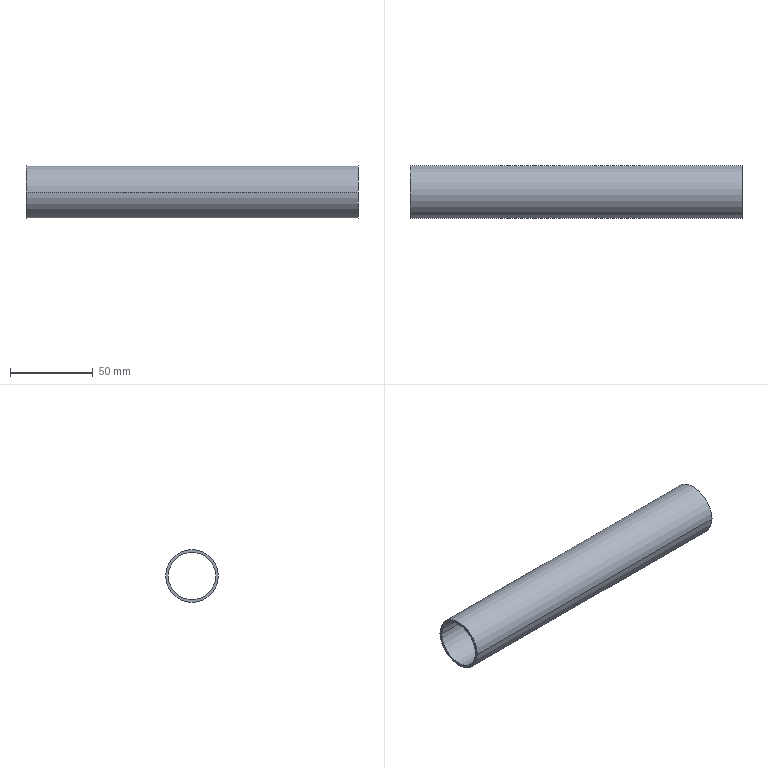Part | NX | features BREP 1 | 1 solid | 6 faces | box 200.025 x 31.75 x 31.75 mm | volume 30090 mm3 | cylinder 4 | plane 2 | commonest cylinder face diameters 28.575 x2 31.75 x2
STEP:
#1=CARTESIAN_POINT('',(-100.013,15.875,0.));
#2=VERTEX_POINT('',#1);
#3=CARTESIAN_POINT('',(-100.013,-15.875,0.));
#4=VERTEX_POINT('',#3);
#5=CARTESIAN_POINT('',(-100.013,0.,0.));
#6=DIRECTION('',(1.,0.,0.));
#7=DIRECTION('',(0.,1.,0.));
#8=AXIS2_PLACEMENT_3D('',#5,#6,#7);
#9=CIRCLE('',#8,15.875);
#10=EDGE_CURVE('',#2,#4,#9,.T.);
#11=ORIENTED_EDGE('',*,*,#10,.F.);
#12=CARTESIAN_POINT('',(-100.013,0.,0.));
#13=DIRECTION('',(1.,0.,0.));
#14=DIRECTION('',(0.,-1.,0.));
#15=AXIS2_PLACEMENT_3D('',#12,#13,#14);
#16=CIRCLE('',#15,15.875);
#17=EDGE_CURVE('',#4,#2,#16,.T.);
#18=ORIENTED_EDGE('',*,*,#17,.F.);
#19=EDGE_LOOP('',(#11,#18));
#20=FACE_BOUND('',#19,.T.);
#21=CARTESIAN_POINT('',(-100.013,14.287,0.));
#22=VERTEX_POINT('',#21);
#23=CARTESIAN_POINT('',(-100.013,-14.287,0.));
#24=VERTEX_POINT('',#23);
#25=CARTESIAN_POINT('',(-100.013,0.,0.));
#26=DIRECTION('',(-1.,0.,0.));
#27=DIRECTION('',(0.,1.,0.));
#28=AXIS2_PLACEMENT_3D('',#25,#26,#27);
#29=CIRCLE('',#28,14.287);
#30=EDGE_CURVE('',#22,#24,#29,.T.);
#31=ORIENTED_EDGE('',*,*,#30,.F.);
#32=CARTESIAN_POINT('',(-100.013,0.,0.));
#33=DIRECTION('',(-1.,0.,0.));
#34=DIRECTION('',(0.,-1.,0.));
#35=AXIS2_PLACEMENT_3D('',#32,#33,#34);
#36=CIRCLE('',#35,14.287);
#37=EDGE_CURVE('',#24,#22,#36,.T.);
#38=ORIENTED_EDGE('',*,*,#37,.F.);
#39=EDGE_LOOP('',(#31,#38));
#40=FACE_BOUND('',#39,.T.);
#41=CARTESIAN_POINT('',(-100.013,0.,0.));
#42=DIRECTION('',(1.,0.,0.));
#43=DIRECTION('',(0.,1.,0.));
#44=AXIS2_PLACEMENT_3D('',#41,#42,#43);
#45=PLANE('',#44);
#46=ADVANCED_FACE('',(#20,#40),#45,.F.);
#47=CARTESIAN_POINT('',(100.013,15.875,0.));
#48=VERTEX_POINT('',#47);
#49=CARTESIAN_POINT('',(-100.013,15.875,0.));
#50=DIRECTION('',(1.,0.,0.));
#51=VECTOR('',#50,1000.);
#52=LINE('',#49,#51);
#53=EDGE_CURVE('',#48,#2,#52,.F.);
#54=ORIENTED_EDGE('',*,*,#53,.F.);
#55=CARTESIAN_POINT('',(100.013,-15.875,0.));
#56=VERTEX_POINT('',#55);
#57=CARTESIAN_POINT('',(100.013,0.,0.));
#58=DIRECTION('',(1.,0.,0.));
#59=DIRECTION('',(0.,-1.,0.));
#60=AXIS2_PLACEMENT_3D('',#57,#58,#59);
#61=CIRCLE('',#60,15.875);
#62=EDGE_CURVE('',#56,#48,#61,.T.);
#63=ORIENTED_EDGE('',*,*,#62,.F.);
#64=CARTESIAN_POINT('',(-100.013,-15.875,0.));
#65=DIRECTION('',(1.,0.,0.));
#66=VECTOR('',#65,1000.);
#67=LINE('',#64,#66);
#68=EDGE_CURVE('',#56,#4,#67,.F.);
#69=ORIENTED_EDGE('',*,*,#68,.T.);
#70=ORIENTED_EDGE('',*,*,#17,.T.);
#71=EDGE_LOOP('',(#54,#63,#69,#70));
#72=FACE_BOUND('',#71,.T.);
#73=CARTESIAN_POINT('',(-100.013,0.,0.));
#74=DIRECTION('',(1.,0.,0.));
#75=DIRECTION('',(0.,-1.,0.));
#76=AXIS2_PLACEMENT_3D('',#73,#74,#75);
#77=CYLINDRICAL_SURFACE('',#76,15.875);
#78=ADVANCED_FACE('',(#72),#77,.T.);
#79=ORIENTED_EDGE('',*,*,#68,.F.);
#80=CARTESIAN_POINT('',(100.013,0.,0.));
#81=DIRECTION('',(1.,0.,0.));
#82=DIRECTION('',(0.,1.,0.));
#83=AXIS2_PLACEMENT_3D('',#80,#81,#82);
#84=CIRCLE('',#83,15.875);
#85=EDGE_CURVE('',#48,#56,#84,.T.);
#86=ORIENTED_EDGE('',*,*,#85,.F.);
#87=ORIENTED_EDGE('',*,*,#53,.T.);
#88=ORIENTED_EDGE('',*,*,#10,.T.);
#89=EDGE_LOOP('',(#79,#86,#87,#88));
#90=FACE_BOUND('',#89,.T.);
#91=CARTESIAN_POINT('',(-100.013,0.,0.));
#92=DIRECTION('',(1.,0.,0.));
#93=DIRECTION('',(0.,-1.,0.));
#94=AXIS2_PLACEMENT_3D('',#91,#92,#93);
#95=CYLINDRICAL_SURFACE('',#94,15.875);
#96=ADVANCED_FACE('',(#90),#95,.T.);
#97=ORIENTED_EDGE('',*,*,#85,.T.);
#98=ORIENTED_EDGE('',*,*,#62,.T.);
#99=EDGE_LOOP('',(#97,#98));
#100=FACE_BOUND('',#99,.T.);
#101=CARTESIAN_POINT('',(100.013,14.287,0.));
#102=VERTEX_POINT('',#101);
#103=CARTESIAN_POINT('',(100.013,-14.287,0.));
#104=VERTEX_POINT('',#103);
#105=CARTESIAN_POINT('',(100.013,0.,0.));
#106=DIRECTION('',(-1.,0.,0.));
#107=DIRECTION('',(0.,1.,0.));
#108=AXIS2_PLACEMENT_3D('',#105,#106,#107);
#109=CIRCLE('',#108,14.287);
#110=EDGE_CURVE('',#102,#104,#109,.T.);
#111=ORIENTED_EDGE('',*,*,#110,.T.);
#112=CARTESIAN_POINT('',(100.013,0.,0.));
#113=DIRECTION('',(-1.,0.,0.));
#114=DIRECTION('',(0.,-1.,0.));
#115=AXIS2_PLACEMENT_3D('',#112,#113,#114);
#116=CIRCLE('',#115,14.287);
#117=EDGE_CURVE('',#104,#102,#116,.T.);
#118=ORIENTED_EDGE('',*,*,#117,.T.);
#119=EDGE_LOOP('',(#111,#118));
#120=FACE_BOUND('',#119,.T.);
#121=CARTESIAN_POINT('',(100.013,0.,0.));
#122=DIRECTION('',(1.,0.,0.));
#123=DIRECTION('',(0.,1.,0.));
#124=AXIS2_PLACEMENT_3D('',#121,#122,#123);
#125=PLANE('',#124);
#126=ADVANCED_FACE('',(#100,#120),#125,.T.);
#127=CARTESIAN_POINT('',(-100.013,14.287,0.));
#128=DIRECTION('',(1.,0.,0.));
#129=VECTOR('',#128,1000.);
#130=LINE('',#127,#129);
#131=EDGE_CURVE('',#102,#22,#130,.F.);
#132=ORIENTED_EDGE('',*,*,#131,.F.);
#133=ORIENTED_EDGE('',*,*,#117,.F.);
#134=CARTESIAN_POINT('',(-100.013,-14.287,0.));
#135=DIRECTION('',(1.,0.,0.));
#136=VECTOR('',#135,1000.);
#137=LINE('',#134,#136);
#138=EDGE_CURVE('',#104,#24,#137,.F.);
#139=ORIENTED_EDGE('',*,*,#138,.T.);
#140=ORIENTED_EDGE('',*,*,#37,.T.);
#141=EDGE_LOOP('',(#132,#133,#139,#140));
#142=FACE_BOUND('',#141,.T.);
#143=CARTESIAN_POINT('',(-100.013,0.,0.));
#144=DIRECTION('',(1.,0.,0.));
#145=DIRECTION('',(0.,-1.,0.));
#146=AXIS2_PLACEMENT_3D('',#143,#144,#145);
#147=CYLINDRICAL_SURFACE('',#146,14.287);
#148=ADVANCED_FACE('',(#142),#147,.F.);
#149=ORIENTED_EDGE('',*,*,#138,.F.);
#150=ORIENTED_EDGE('',*,*,#110,.F.);
#151=ORIENTED_EDGE('',*,*,#131,.T.);
#152=ORIENTED_EDGE('',*,*,#30,.T.);
#153=EDGE_LOOP('',(#149,#150,#151,#152));
#154=FACE_BOUND('',#153,.T.);
#155=CARTESIAN_POINT('',(-100.013,0.,0.));
#156=DIRECTION('',(1.,0.,0.));
#157=DIRECTION('',(0.,-1.,0.));
#158=AXIS2_PLACEMENT_3D('',#155,#156,#157);
#159=CYLINDRICAL_SURFACE('',#158,14.287);
#160=ADVANCED_FACE('',(#154),#159,.F.);
#161=CLOSED_SHELL('',(#46,#78,#96,#126,#148,#160));
#162=MANIFOLD_SOLID_BREP('',#161);
#163=(LENGTH_UNIT()NAMED_UNIT(*)SI_UNIT(.MILLI.,.METRE.));
#164=UNCERTAINTY_MEASURE_WITH_UNIT(LENGTH_MEASURE(0.00001),#163,'','');
#165=(NAMED_UNIT(*)PLANE_ANGLE_UNIT()SI_UNIT($,.RADIAN.));
#166=(NAMED_UNIT(*)SI_UNIT($,.STERADIAN.)SOLID_ANGLE_UNIT());
#167=(GEOMETRIC_REPRESENTATION_CONTEXT(3)GLOBAL_UNCERTAINTY_ASSIGNED_CONTEXT((#164))GLOBAL_UNIT_ASSIGNED_CONTEXT((#163,#165,#166))REPRESENTATION_CONTEXT('',''));
#168=ADVANCED_BREP_SHAPE_REPRESENTATION('',(#162),#167);